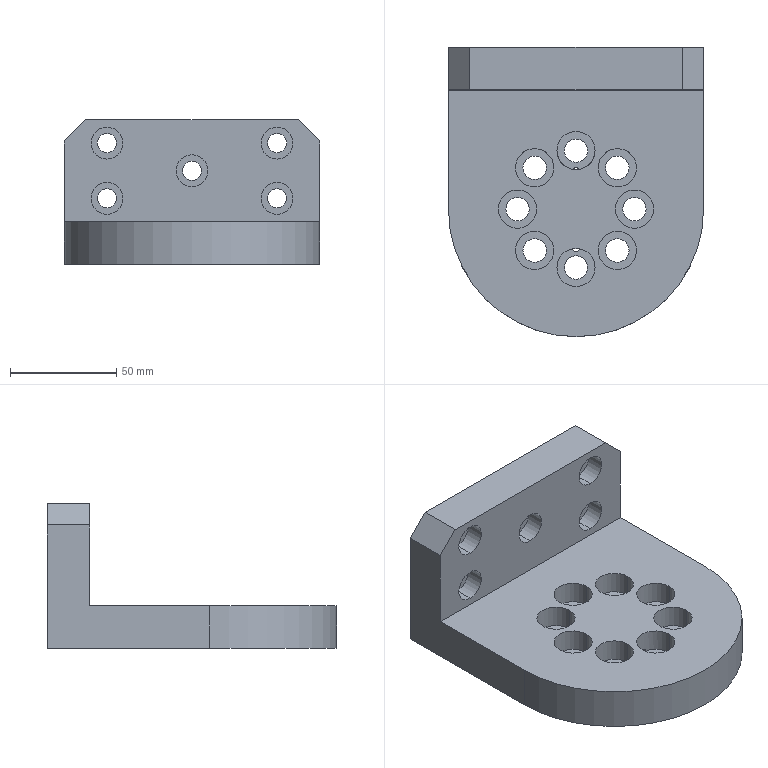Part | SolidWorks | features HoleWzd 4, Chamfer 1, Extrusion 1, ICE 1 | 1 solid | 87 faces | box 120 x 136 x 68 mm | volume 368287 mm3 | cylinder 57 | plane 26 | cone 4 | commonest cylinder face diameters 11 x16 18 x16 9 x10 15 x10 5 x4 120 x1